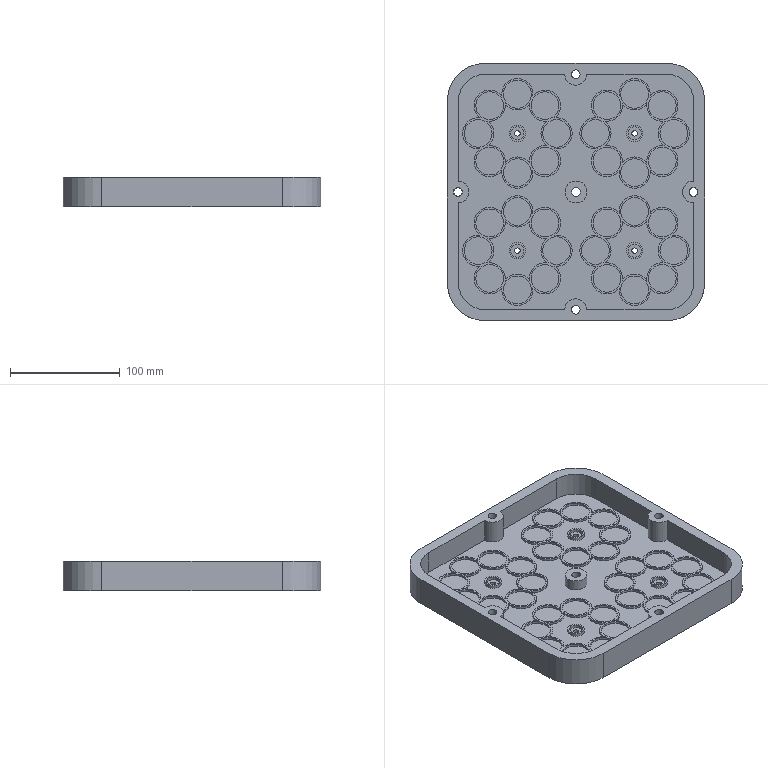Part | SolidWorks | features ICE 4, Extrusion 1 | 1 solid | 299 faces | box 235 x 235 x 27 mm | volume 476715 mm3 | cylinder 227 | plane 72 | commonest cylinder face diameters 28.5 x104 25.4 x64 8 x18 20 x9 5 x8 12 x8